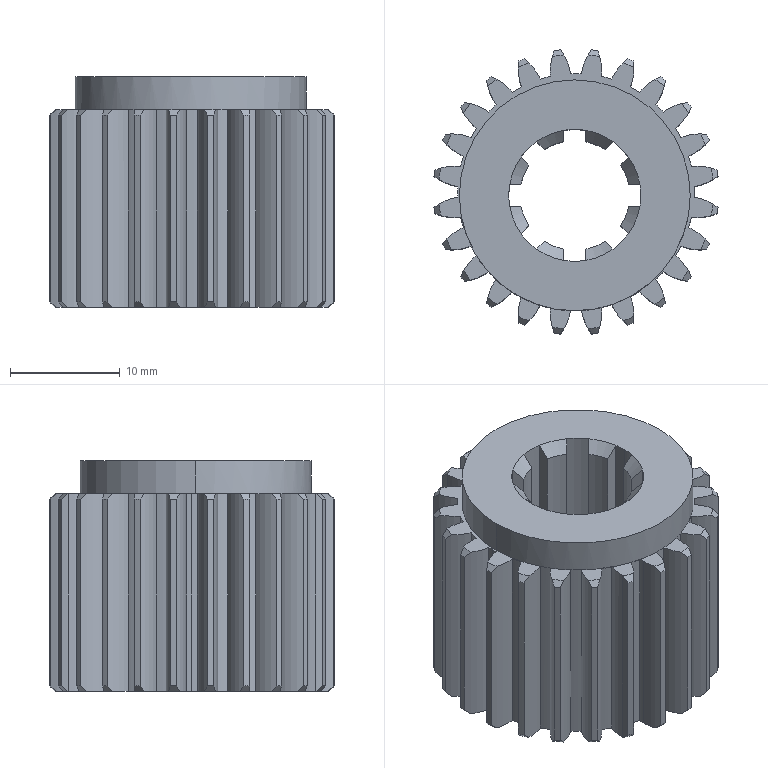Part | SolidWorks | features Chamfer 3, ICE 2, Extrusion 1 | 1 solid | 206 faces | box 25.844 x 25.844 x 21 mm | volume 6942 mm3 | cylinder 120 | cone 56 | plane 30 | commonest cylinder face diameters 9.6 x52 21.498 x25 26 x24 12 x9 10 x8 21 x2